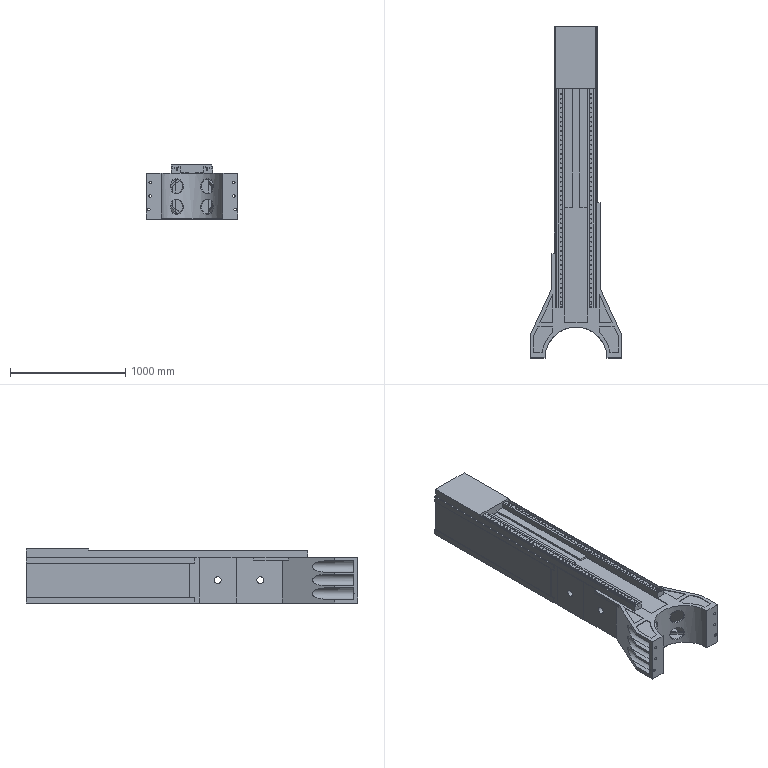Part | STEP file | Boss-Extrude 52 | 1 solid | 974 faces | box 790 x 2874 x 468.842 mm | volume 233338953 mm3 | plane 439 | cylinder 338 | cone 197 | commonest cylinder face diameters 6.8 x192 85 x24 70 x16 20 x12 22 x12 38 x12